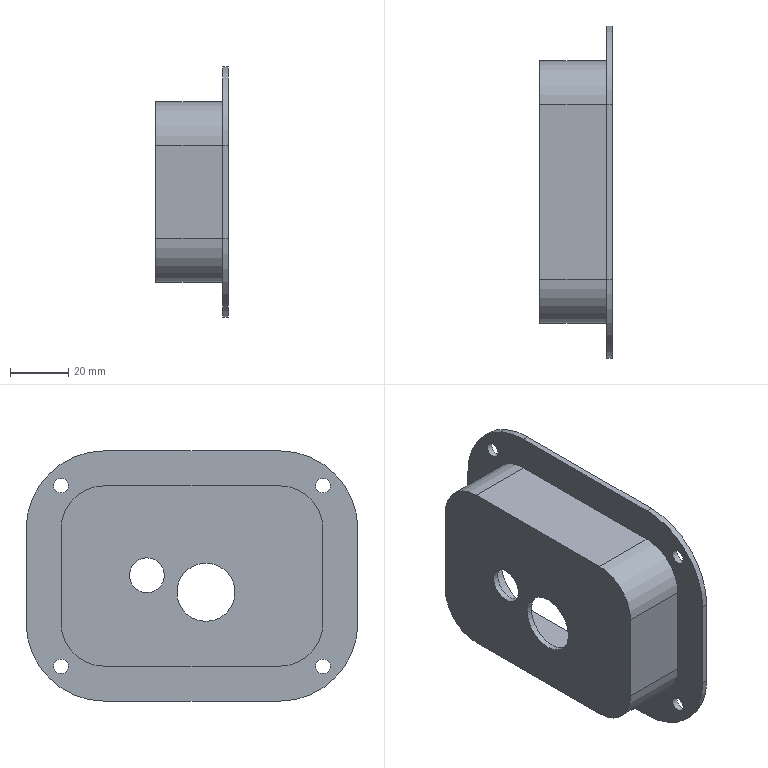Part | STEP file | Plug | 1 solid | 34 faces | box 25 x 114 x 86 mm | volume 29855 mm3 | cylinder 18 | plane 16 | commonest cylinder face diameters 5 x4 26 x4 30 x4 54 x4 12 x1 20 x1
STEP:
#1=CARTESIAN_POINT('',(23.,102.,-15.));
#2=VERTEX_POINT('',#1);
#3=CARTESIAN_POINT('',(23.,75.,12.));
#4=VERTEX_POINT('',#3);
#5=CARTESIAN_POINT('',(23.,75.,-15.));
#6=DIRECTION('',(1.,0.,0.));
#7=DIRECTION('',(0.,1.,0.));
#8=AXIS2_PLACEMENT_3D('',#5,#6,#7);
#9=CIRCLE('',#8,27.);
#10=EDGE_CURVE('',#2,#4,#9,.T.);
#11=ORIENTED_EDGE('',*,*,#10,.F.);
#12=CARTESIAN_POINT('',(23.,102.,-47.));
#13=VERTEX_POINT('',#12);
#14=CARTESIAN_POINT('',(23.,102.,-47.));
#15=DIRECTION('',(0.,0.,1.));
#16=VECTOR('',#15,1.);
#17=LINE('',#14,#16);
#18=EDGE_CURVE('',#13,#2,#17,.T.);
#19=ORIENTED_EDGE('',*,*,#18,.F.);
#20=CARTESIAN_POINT('',(23.,75.,-74.));
#21=VERTEX_POINT('',#20);
#22=CARTESIAN_POINT('',(23.,75.,-47.));
#23=DIRECTION('',(1.,0.,0.));
#24=DIRECTION('',(0.,0.,-1.));
#25=AXIS2_PLACEMENT_3D('',#22,#23,#24);
#26=CIRCLE('',#25,27.);
#27=EDGE_CURVE('',#21,#13,#26,.T.);
#28=ORIENTED_EDGE('',*,*,#27,.F.);
#29=CARTESIAN_POINT('',(23.,15.,-74.));
#30=VERTEX_POINT('',#29);
#31=CARTESIAN_POINT('',(23.,15.,-74.));
#32=DIRECTION('',(0.,1.,0.));
#33=VECTOR('',#32,1.);
#34=LINE('',#31,#33);
#35=EDGE_CURVE('',#30,#21,#34,.T.);
#36=ORIENTED_EDGE('',*,*,#35,.F.);
#37=CARTESIAN_POINT('',(23.,-12.,-47.));
#38=VERTEX_POINT('',#37);
#39=CARTESIAN_POINT('',(23.,15.,-47.));
#40=DIRECTION('',(1.,0.,0.));
#41=DIRECTION('',(0.,-1.,0.));
#42=AXIS2_PLACEMENT_3D('',#39,#40,#41);
#43=CIRCLE('',#42,27.);
#44=EDGE_CURVE('',#38,#30,#43,.T.);
#45=ORIENTED_EDGE('',*,*,#44,.F.);
#46=CARTESIAN_POINT('',(23.,-12.,-15.));
#47=VERTEX_POINT('',#46);
#48=CARTESIAN_POINT('',(23.,-12.,-15.));
#49=DIRECTION('',(0.,0.,-1.));
#50=VECTOR('',#49,1.);
#51=LINE('',#48,#50);
#52=EDGE_CURVE('',#47,#38,#51,.T.);
#53=ORIENTED_EDGE('',*,*,#52,.F.);
#54=CARTESIAN_POINT('',(23.,15.,12.));
#55=VERTEX_POINT('',#54);
#56=CARTESIAN_POINT('',(23.,15.,-15.));
#57=DIRECTION('',(1.,0.,0.));
#58=DIRECTION('',(0.,0.,1.));
#59=AXIS2_PLACEMENT_3D('',#56,#57,#58);
#60=CIRCLE('',#59,27.);
#61=EDGE_CURVE('',#55,#47,#60,.T.);
#62=ORIENTED_EDGE('',*,*,#61,.F.);
#63=CARTESIAN_POINT('',(23.,75.,12.));
#64=DIRECTION('',(0.,-1.,0.));
#65=VECTOR('',#64,1.);
#66=LINE('',#63,#65);
#67=EDGE_CURVE('',#4,#55,#66,.T.);
#68=ORIENTED_EDGE('',*,*,#67,.F.);
#69=EDGE_LOOP('',(#11,#19,#28,#36,#45,#53,#62,#68));
#70=FACE_BOUND('',#69,.T.);
#71=CARTESIAN_POINT('',(23.,92.5,-62.));
#72=VERTEX_POINT('',#71);
#73=CARTESIAN_POINT('',(23.,90.,-62.));
#74=DIRECTION('',(1.,0.,0.));
#75=DIRECTION('',(0.,1.,0.));
#76=AXIS2_PLACEMENT_3D('',#73,#74,#75);
#77=CIRCLE('',#76,2.5);
#78=EDGE_CURVE('',#72,#72,#77,.T.);
#79=ORIENTED_EDGE('',*,*,#78,.T.);
#80=EDGE_LOOP('',(#79));
#81=FACE_BOUND('',#80,.T.);
#82=CARTESIAN_POINT('',(23.,2.5,-62.));
#83=VERTEX_POINT('',#82);
#84=CARTESIAN_POINT('',(23.,0.,-62.));
#85=DIRECTION('',(1.,0.,0.));
#86=DIRECTION('',(0.,1.,0.));
#87=AXIS2_PLACEMENT_3D('',#84,#85,#86);
#88=CIRCLE('',#87,2.5);
#89=EDGE_CURVE('',#83,#83,#88,.T.);
#90=ORIENTED_EDGE('',*,*,#89,.T.);
#91=EDGE_LOOP('',(#90));
#92=FACE_BOUND('',#91,.T.);
#93=CARTESIAN_POINT('',(23.,2.5,0.));
#94=VERTEX_POINT('',#93);
#95=CARTESIAN_POINT('',(23.,0.,0.));
#96=DIRECTION('',(1.,0.,0.));
#97=DIRECTION('',(0.,1.,0.));
#98=AXIS2_PLACEMENT_3D('',#95,#96,#97);
#99=CIRCLE('',#98,2.5);
#100=EDGE_CURVE('',#94,#94,#99,.T.);
#101=ORIENTED_EDGE('',*,*,#100,.T.);
#102=EDGE_LOOP('',(#101));
#103=FACE_BOUND('',#102,.T.);
#104=CARTESIAN_POINT('',(23.,0.,-47.));
#105=VERTEX_POINT('',#104);
#106=CARTESIAN_POINT('',(23.,15.,-62.));
#107=VERTEX_POINT('',#106);
#108=CARTESIAN_POINT('',(23.,15.,-47.));
#109=DIRECTION('',(-1.,0.,0.));
#110=DIRECTION('',(0.,0.,-1.));
#111=AXIS2_PLACEMENT_3D('',#108,#109,#110);
#112=CIRCLE('',#111,15.);
#113=EDGE_CURVE('',#105,#107,#112,.F.);
#114=ORIENTED_EDGE('',*,*,#113,.T.);
#115=CARTESIAN_POINT('',(23.,75.,-62.));
#116=VERTEX_POINT('',#115);
#117=CARTESIAN_POINT('',(23.,75.,-62.));
#118=DIRECTION('',(0.,-1.,0.));
#119=VECTOR('',#118,1.);
#120=LINE('',#117,#119);
#121=EDGE_CURVE('',#107,#116,#120,.F.);
#122=ORIENTED_EDGE('',*,*,#121,.T.);
#123=CARTESIAN_POINT('',(23.,90.,-47.));
#124=VERTEX_POINT('',#123);
#125=CARTESIAN_POINT('',(23.,75.,-47.));
#126=DIRECTION('',(-1.,0.,0.));
#127=DIRECTION('',(0.,1.,0.));
#128=AXIS2_PLACEMENT_3D('',#125,#126,#127);
#129=CIRCLE('',#128,15.);
#130=EDGE_CURVE('',#116,#124,#129,.F.);
#131=ORIENTED_EDGE('',*,*,#130,.T.);
#132=CARTESIAN_POINT('',(23.,90.,-15.));
#133=VERTEX_POINT('',#132);
#134=CARTESIAN_POINT('',(23.,90.,-15.));
#135=DIRECTION('',(0.,0.,-1.));
#136=VECTOR('',#135,1.);
#137=LINE('',#134,#136);
#138=EDGE_CURVE('',#124,#133,#137,.F.);
#139=ORIENTED_EDGE('',*,*,#138,.T.);
#140=CARTESIAN_POINT('',(23.,75.,0.));
#141=VERTEX_POINT('',#140);
#142=CARTESIAN_POINT('',(23.,75.,-15.));
#143=DIRECTION('',(-1.,0.,0.));
#144=DIRECTION('',(0.,0.,1.));
#145=AXIS2_PLACEMENT_3D('',#142,#143,#144);
#146=CIRCLE('',#145,15.);
#147=EDGE_CURVE('',#133,#141,#146,.F.);
#148=ORIENTED_EDGE('',*,*,#147,.T.);
#149=CARTESIAN_POINT('',(23.,15.,0.));
#150=VERTEX_POINT('',#149);
#151=CARTESIAN_POINT('',(23.,15.,0.));
#152=DIRECTION('',(0.,1.,0.));
#153=VECTOR('',#152,1.);
#154=LINE('',#151,#153);
#155=EDGE_CURVE('',#141,#150,#154,.F.);
#156=ORIENTED_EDGE('',*,*,#155,.T.);
#157=CARTESIAN_POINT('',(23.,0.,-15.));
#158=VERTEX_POINT('',#157);
#159=CARTESIAN_POINT('',(23.,15.,-15.));
#160=DIRECTION('',(-1.,0.,0.));
#161=DIRECTION('',(0.,-1.,0.));
#162=AXIS2_PLACEMENT_3D('',#159,#160,#161);
#163=CIRCLE('',#162,15.);
#164=EDGE_CURVE('',#150,#158,#163,.F.);
#165=ORIENTED_EDGE('',*,*,#164,.T.);
#166=CARTESIAN_POINT('',(23.,0.,-47.));
#167=DIRECTION('',(0.,0.,1.));
#168=VECTOR('',#167,1.);
#169=LINE('',#166,#168);
#170=EDGE_CURVE('',#158,#105,#169,.F.);
#171=ORIENTED_EDGE('',*,*,#170,.T.);
#172=EDGE_LOOP('',(#114,#122,#131,#139,#148,#156,#165,#171));
#173=FACE_BOUND('',#172,.T.);
#174=CARTESIAN_POINT('',(23.,92.5,0.));
#175=VERTEX_POINT('',#174);
#176=CARTESIAN_POINT('',(23.,90.,0.));
#177=DIRECTION('',(1.,0.,0.));
#178=DIRECTION('',(0.,1.,0.));
#179=AXIS2_PLACEMENT_3D('',#176,#177,#178);
#180=CIRCLE('',#179,2.5);
#181=EDGE_CURVE('',#175,#175,#180,.T.);
#182=ORIENTED_EDGE('',*,*,#181,.T.);
#183=EDGE_LOOP('',(#182));
#184=FACE_BOUND('',#183,.T.);
#185=CARTESIAN_POINT('',(23.,0.,0.));
#186=DIRECTION('',(1.,0.,0.));
#187=DIRECTION('',(0.,0.,-1.));
#188=AXIS2_PLACEMENT_3D('',#185,#186,#187);
#189=PLANE('',#188);
#190=ADVANCED_FACE('',(#70,#81,#92,#103,#173,#184),#189,.F.);
#191=CARTESIAN_POINT('',(25.,75.,12.));
#192=VERTEX_POINT('',#191);
#193=CARTESIAN_POINT('',(25.,15.,12.));
#194=VERTEX_POINT('',#193);
#195=CARTESIAN_POINT('',(25.,75.,12.));
#196=DIRECTION('',(0.,-1.,0.));
#197=VECTOR('',#196,1.);
#198=LINE('',#195,#197);
#199=EDGE_CURVE('',#192,#194,#198,.T.);
#200=ORIENTED_EDGE('',*,*,#199,.T.);
#201=CARTESIAN_POINT('',(25.,-12.,-15.));
#202=VERTEX_POINT('',#201);
#203=CARTESIAN_POINT('',(25.,15.,-15.));
#204=DIRECTION('',(1.,0.,0.));
#205=DIRECTION('',(0.,0.,1.));
#206=AXIS2_PLACEMENT_3D('',#203,#204,#205);
#207=CIRCLE('',#206,27.);
#208=EDGE_CURVE('',#194,#202,#207,.T.);
#209=ORIENTED_EDGE('',*,*,#208,.T.);
#210=CARTESIAN_POINT('',(25.,-12.,-47.));
#211=VERTEX_POINT('',#210);
#212=CARTESIAN_POINT('',(25.,-12.,-15.));
#213=DIRECTION('',(0.,0.,-1.));
#214=VECTOR('',#213,1.);
#215=LINE('',#212,#214);
#216=EDGE_CURVE('',#202,#211,#215,.T.);
#217=ORIENTED_EDGE('',*,*,#216,.T.);
#218=CARTESIAN_POINT('',(25.,15.,-74.));
#219=VERTEX_POINT('',#218);
#220=CARTESIAN_POINT('',(25.,15.,-47.));
#221=DIRECTION('',(1.,0.,0.));
#222=DIRECTION('',(0.,-1.,0.));
#223=AXIS2_PLACEMENT_3D('',#220,#221,#222);
#224=CIRCLE('',#223,27.);
#225=EDGE_CURVE('',#211,#219,#224,.T.);
#226=ORIENTED_EDGE('',*,*,#225,.T.);
#227=CARTESIAN_POINT('',(25.,75.,-74.));
#228=VERTEX_POINT('',#227);
#229=CARTESIAN_POINT('',(25.,15.,-74.));
#230=DIRECTION('',(0.,1.,0.));
#231=VECTOR('',#230,1.);
#232=LINE('',#229,#231);
#233=EDGE_CURVE('',#219,#228,#232,.T.);
#234=ORIENTED_EDGE('',*,*,#233,.T.);
#235=CARTESIAN_POINT('',(25.,102.,-47.));
#236=VERTEX_POINT('',#235);
#237=CARTESIAN_POINT('',(25.,75.,-47.));
#238=DIRECTION('',(1.,0.,0.));
#239=DIRECTION('',(0.,0.,-1.));
#240=AXIS2_PLACEMENT_3D('',#237,#238,#239);
#241=CIRCLE('',#240,27.);
#242=EDGE_CURVE('',#228,#236,#241,.T.);
#243=ORIENTED_EDGE('',*,*,#242,.T.);
#244=CARTESIAN_POINT('',(25.,102.,-15.));
#245=VERTEX_POINT('',#244);
#246=CARTESIAN_POINT('',(25.,102.,-47.));
#247=DIRECTION('',(0.,0.,1.));
#248=VECTOR('',#247,1.);
#249=LINE('',#246,#248);
#250=EDGE_CURVE('',#236,#245,#249,.T.);
#251=ORIENTED_EDGE('',*,*,#250,.T.);
#252=CARTESIAN_POINT('',(25.,75.,-15.));
#253=DIRECTION('',(1.,0.,0.));
#254=DIRECTION('',(0.,1.,0.));
#255=AXIS2_PLACEMENT_3D('',#252,#253,#254);
#256=CIRCLE('',#255,27.);
#257=EDGE_CURVE('',#245,#192,#256,.T.);
#258=ORIENTED_EDGE('',*,*,#257,.T.);
#259=EDGE_LOOP('',(#200,#209,#217,#226,#234,#243,#251,#258));
#260=FACE_BOUND('',#259,.T.);
#261=CARTESIAN_POINT('',(25.,92.5,-62.));
#262=VERTEX_POINT('',#261);
#263=CARTESIAN_POINT('',(25.,90.,-62.));
#264=DIRECTION('',(1.,0.,0.));
#265=DIRECTION('',(0.,1.,0.));
#266=AXIS2_PLACEMENT_3D('',#263,#264,#265);
#267=CIRCLE('',#266,2.5);
#268=EDGE_CURVE('',#262,#262,#267,.F.);
#269=ORIENTED_EDGE('',*,*,#268,.T.);
#270=EDGE_LOOP('',(#269));
#271=FACE_BOUND('',#270,.T.);
#272=CARTESIAN_POINT('',(25.,2.5,-62.));
#273=VERTEX_POINT('',#272);
#274=CARTESIAN_POINT('',(25.,0.,-62.));
#275=DIRECTION('',(1.,0.,0.));
#276=DIRECTION('',(0.,1.,0.));
#277=AXIS2_PLACEMENT_3D('',#274,#275,#276);
#278=CIRCLE('',#277,2.5);
#279=EDGE_CURVE('',#273,#273,#278,.F.);
#280=ORIENTED_EDGE('',*,*,#279,.T.);
#281=EDGE_LOOP('',(#280));
#282=FACE_BOUND('',#281,.T.);
#283=CARTESIAN_POINT('',(25.,2.5,0.));
#284=VERTEX_POINT('',#283);
#285=CARTESIAN_POINT('',(25.,0.,0.));
#286=DIRECTION('',(1.,0.,0.));
#287=DIRECTION('',(0.,1.,0.));
#288=AXIS2_PLACEMENT_3D('',#285,#286,#287);
#289=CIRCLE('',#288,2.5);
#290=EDGE_CURVE('',#284,#284,#289,.F.);
#291=ORIENTED_EDGE('',*,*,#290,.T.);
#292=EDGE_LOOP('',(#291));
#293=FACE_BOUND('',#292,.T.);
#294=CARTESIAN_POINT('',(25.,75.,-2.));
#295=VERTEX_POINT('',#294);
#296=CARTESIAN_POINT('',(25.,88.,-15.));
#297=VERTEX_POINT('',#296);
#298=CARTESIAN_POINT('',(25.,75.,-15.));
#299=DIRECTION('',(1.,0.,0.));
#300=DIRECTION('',(0.,1.,0.));
#301=AXIS2_PLACEMENT_3D('',#298,#299,#300);
#302=CIRCLE('',#301,13.);
#303=EDGE_CURVE('',#295,#297,#302,.F.);
#304=ORIENTED_EDGE('',*,*,#303,.T.);
#305=CARTESIAN_POINT('',(25.,88.,-47.));
#306=VERTEX_POINT('',#305);
#307=CARTESIAN_POINT('',(25.,88.,-47.));
#308=DIRECTION('',(0.,0.,1.));
#309=VECTOR('',#308,1.);
#310=LINE('',#307,#309);
#311=EDGE_CURVE('',#297,#306,#310,.F.);
#312=ORIENTED_EDGE('',*,*,#311,.T.);
#313=CARTESIAN_POINT('',(25.,75.,-60.));
#314=VERTEX_POINT('',#313);
#315=CARTESIAN_POINT('',(25.,75.,-47.));
#316=DIRECTION('',(1.,0.,0.));
#317=DIRECTION('',(0.,0.,-1.));
#318=AXIS2_PLACEMENT_3D('',#315,#316,#317);
#319=CIRCLE('',#318,13.);
#320=EDGE_CURVE('',#306,#314,#319,.F.);
#321=ORIENTED_EDGE('',*,*,#320,.T.);
#322=CARTESIAN_POINT('',(25.,15.,-60.));
#323=VERTEX_POINT('',#322);
#324=CARTESIAN_POINT('',(25.,15.,-60.));
#325=DIRECTION('',(0.,1.,0.));
#326=VECTOR('',#325,1.);
#327=LINE('',#324,#326);
#328=EDGE_CURVE('',#314,#323,#327,.F.);
#329=ORIENTED_EDGE('',*,*,#328,.T.);
#330=CARTESIAN_POINT('',(25.,2.,-47.));
#331=VERTEX_POINT('',#330);
#332=CARTESIAN_POINT('',(25.,15.,-47.));
#333=DIRECTION('',(1.,0.,0.));
#334=DIRECTION('',(0.,-1.,0.));
#335=AXIS2_PLACEMENT_3D('',#332,#333,#334);
#336=CIRCLE('',#335,13.);
#337=EDGE_CURVE('',#323,#331,#336,.F.);
#338=ORIENTED_EDGE('',*,*,#337,.T.);
#339=CARTESIAN_POINT('',(25.,2.,-15.));
#340=VERTEX_POINT('',#339);
#341=CARTESIAN_POINT('',(25.,2.,-15.));
#342=DIRECTION('',(0.,0.,-1.));
#343=VECTOR('',#342,1.);
#344=LINE('',#341,#343);
#345=EDGE_CURVE('',#331,#340,#344,.F.);
#346=ORIENTED_EDGE('',*,*,#345,.T.);
#347=CARTESIAN_POINT('',(25.,15.,-2.));
#348=VERTEX_POINT('',#347);
#349=CARTESIAN_POINT('',(25.,15.,-15.));
#350=DIRECTION('',(1.,0.,0.));
#351=DIRECTION('',(0.,0.,1.));
#352=AXIS2_PLACEMENT_3D('',#349,#350,#351);
#353=CIRCLE('',#352,13.);
#354=EDGE_CURVE('',#340,#348,#353,.F.);
#355=ORIENTED_EDGE('',*,*,#354,.T.);
#356=CARTESIAN_POINT('',(25.,75.,-2.));
#357=DIRECTION('',(0.,-1.,0.));
#358=VECTOR('',#357,1.);
#359=LINE('',#356,#358);
#360=EDGE_CURVE('',#348,#295,#359,.F.);
#361=ORIENTED_EDGE('',*,*,#360,.T.);
#362=EDGE_LOOP('',(#304,#312,#321,#329,#338,#346,#355,#361));
#363=FACE_BOUND('',#362,.T.);
#364=CARTESIAN_POINT('',(25.,92.5,0.));
#365=VERTEX_POINT('',#364);
#366=CARTESIAN_POINT('',(25.,90.,0.));
#367=DIRECTION('',(1.,0.,0.));
#368=DIRECTION('',(0.,1.,0.));
#369=AXIS2_PLACEMENT_3D('',#366,#367,#368);
#370=CIRCLE('',#369,2.5);
#371=EDGE_CURVE('',#365,#365,#370,.F.);
#372=ORIENTED_EDGE('',*,*,#371,.T.);
#373=EDGE_LOOP('',(#372));
#374=FACE_BOUND('',#373,.T.);
#375=CARTESIAN_POINT('',(25.,0.,0.));
#376=DIRECTION('',(1.,0.,0.));
#377=DIRECTION('',(0.,0.,-1.));
#378=AXIS2_PLACEMENT_3D('',#375,#376,#377);
#379=PLANE('',#378);
#380=ADVANCED_FACE('',(#260,#271,#282,#293,#363,#374),#379,.T.);
#381=ORIENTED_EDGE('',*,*,#290,.F.);
#382=EDGE_LOOP('',(#381));
#383=FACE_OUTER_BOUND('',#382,.T.);
#384=ORIENTED_EDGE('',*,*,#100,.F.);
#385=EDGE_LOOP('',(#384));
#386=FACE_OUTER_BOUND('',#385,.T.);
#387=CARTESIAN_POINT('',(-15.,0.,0.));
#388=DIRECTION('',(1.,0.,0.));
#389=DIRECTION('',(0.,1.,0.));
#390=AXIS2_PLACEMENT_3D('',#387,#388,#389);
#391=CYLINDRICAL_SURFACE('',#390,2.5);
#392=ADVANCED_FACE('',(#383,#386),#391,.F.);
#393=ORIENTED_EDGE('',*,*,#279,.F.);
#394=EDGE_LOOP('',(#393));
#395=FACE_OUTER_BOUND('',#394,.T.);
#396=ORIENTED_EDGE('',*,*,#89,.F.);
#397=EDGE_LOOP('',(#396));
#398=FACE_OUTER_BOUND('',#397,.T.);
#399=CARTESIAN_POINT('',(-15.,0.,-62.));
#400=DIRECTION('',(1.,0.,0.));
#401=DIRECTION('',(0.,1.,0.));
#402=AXIS2_PLACEMENT_3D('',#399,#400,#401);
#403=CYLINDRICAL_SURFACE('',#402,2.5);
#404=ADVANCED_FACE('',(#395,#398),#403,.F.);
#405=ORIENTED_EDGE('',*,*,#268,.F.);
#406=EDGE_LOOP('',(#405));
#407=FACE_OUTER_BOUND('',#406,.T.);
#408=ORIENTED_EDGE('',*,*,#78,.F.);
#409=EDGE_LOOP('',(#408));
#410=FACE_OUTER_BOUND('',#409,.T.);
#411=CARTESIAN_POINT('',(-15.,90.,-62.));
#412=DIRECTION('',(1.,0.,0.));
#413=DIRECTION('',(0.,1.,0.));
#414=AXIS2_PLACEMENT_3D('',#411,#412,#413);
#415=CYLINDRICAL_SURFACE('',#414,2.5);
#416=ADVANCED_FACE('',(#407,#410),#415,.F.);
#417=ORIENTED_EDGE('',*,*,#10,.T.);
#418=CARTESIAN_POINT('',(23.,75.,12.));
#419=DIRECTION('',(1.,0.,0.));
#420=VECTOR('',#419,1.);
#421=LINE('',#418,#420);
#422=EDGE_CURVE('',#4,#192,#421,.T.);
#423=ORIENTED_EDGE('',*,*,#422,.T.);
#424=ORIENTED_EDGE('',*,*,#257,.F.);
#425=CARTESIAN_POINT('',(23.,102.,-15.));
#426=DIRECTION('',(1.,0.,0.));
#427=VECTOR('',#426,1.);
#428=LINE('',#425,#427);
#429=EDGE_CURVE('',#2,#245,#428,.T.);
#430=ORIENTED_EDGE('',*,*,#429,.F.);
#431=EDGE_LOOP('',(#417,#423,#424,#430));
#432=FACE_BOUND('',#431,.T.);
#433=CARTESIAN_POINT('',(23.,75.,-15.));
#434=DIRECTION('',(1.,0.,0.));
#435=DIRECTION('',(0.,1.,0.));
#436=AXIS2_PLACEMENT_3D('',#433,#434,#435);
#437=CYLINDRICAL_SURFACE('',#436,27.);
#438=ADVANCED_FACE('',(#432),#437,.T.);
#439=ORIENTED_EDGE('',*,*,#18,.T.);
#440=ORIENTED_EDGE('',*,*,#429,.T.);
#441=ORIENTED_EDGE('',*,*,#250,.F.);
#442=CARTESIAN_POINT('',(23.,102.,-47.));
#443=DIRECTION('',(1.,0.,0.));
#444=VECTOR('',#443,1.);
#445=LINE('',#442,#444);
#446=EDGE_CURVE('',#13,#236,#445,.T.);
#447=ORIENTED_EDGE('',*,*,#446,.F.);
#448=EDGE_LOOP('',(#439,#440,#441,#447));
#449=FACE_BOUND('',#448,.T.);
#450=CARTESIAN_POINT('',(23.,102.,-47.));
#451=DIRECTION('',(0.,1.,0.));
#452=DIRECTION('',(0.,0.,1.));
#453=AXIS2_PLACEMENT_3D('',#450,#451,#452);
#454=PLANE('',#453);
#455=ADVANCED_FACE('',(#449),#454,.T.);
#456=ORIENTED_EDGE('',*,*,#27,.T.);
#457=ORIENTED_EDGE('',*,*,#446,.T.);
#458=ORIENTED_EDGE('',*,*,#242,.F.);
#459=CARTESIAN_POINT('',(23.,75.,-74.));
#460=DIRECTION('',(1.,0.,0.));
#461=VECTOR('',#460,1.);
#462=LINE('',#459,#461);
#463=EDGE_CURVE('',#21,#228,#462,.T.);
#464=ORIENTED_EDGE('',*,*,#463,.F.);
#465=EDGE_LOOP('',(#456,#457,#458,#464));
#466=FACE_BOUND('',#465,.T.);
#467=CARTESIAN_POINT('',(23.,75.,-47.));
#468=DIRECTION('',(1.,0.,0.));
#469=DIRECTION('',(0.,0.,-1.));
#470=AXIS2_PLACEMENT_3D('',#467,#468,#469);
#471=CYLINDRICAL_SURFACE('',#470,27.);
#472=ADVANCED_FACE('',(#466),#471,.T.);
#473=ORIENTED_EDGE('',*,*,#35,.T.);
#474=ORIENTED_EDGE('',*,*,#463,.T.);
#475=ORIENTED_EDGE('',*,*,#233,.F.);
#476=CARTESIAN_POINT('',(23.,15.,-74.));
#477=DIRECTION('',(1.,0.,0.));
#478=VECTOR('',#477,1.);
#479=LINE('',#476,#478);
#480=EDGE_CURVE('',#30,#219,#479,.T.);
#481=ORIENTED_EDGE('',*,*,#480,.F.);
#482=EDGE_LOOP('',(#473,#474,#475,#481));
#483=FACE_BOUND('',#482,.T.);
#484=CARTESIAN_POINT('',(23.,15.,-74.));
#485=DIRECTION('',(0.,0.,-1.));
#486=DIRECTION('',(0.,1.,0.));
#487=AXIS2_PLACEMENT_3D('',#484,#485,#486);
#488=PLANE('',#487);
#489=ADVANCED_FACE('',(#483),#488,.T.);
#490=ORIENTED_EDGE('',*,*,#44,.T.);
#491=ORIENTED_EDGE('',*,*,#480,.T.);
#492=ORIENTED_EDGE('',*,*,#225,.F.);
#493=CARTESIAN_POINT('',(23.,-12.,-47.));
#494=DIRECTION('',(1.,0.,0.));
#495=VECTOR('',#494,1.);
#496=LINE('',#493,#495);
#497=EDGE_CURVE('',#38,#211,#496,.T.);
#498=ORIENTED_EDGE('',*,*,#497,.F.);
#499=EDGE_LOOP('',(#490,#491,#492,#498));
#500=FACE_BOUND('',#499,.T.);
#501=CARTESIAN_POINT('',(23.,15.,-47.));
#502=DIRECTION('',(1.,0.,0.));
#503=DIRECTION('',(0.,-1.,0.));
#504=AXIS2_PLACEMENT_3D('',#501,#502,#503);
#505=CYLINDRICAL_SURFACE('',#504,27.);
#506=ADVANCED_FACE('',(#500),#505,.T.);
#507=ORIENTED_EDGE('',*,*,#52,.T.);
#508=ORIENTED_EDGE('',*,*,#497,.T.);
#509=ORIENTED_EDGE('',*,*,#216,.F.);
#510=CARTESIAN_POINT('',(23.,-12.,-15.));
#511=DIRECTION('',(1.,0.,0.));
#512=VECTOR('',#511,1.);
#513=LINE('',#510,#512);
#514=EDGE_CURVE('',#47,#202,#513,.T.);
#515=ORIENTED_EDGE('',*,*,#514,.F.);
#516=EDGE_LOOP('',(#507,#508,#509,#515));
#517=FACE_BOUND('',#516,.T.);
#518=CARTESIAN_POINT('',(23.,-12.,-15.));
#519=DIRECTION('',(0.,-1.,0.));
#520=DIRECTION('',(0.,0.,-1.));
#521=AXIS2_PLACEMENT_3D('',#518,#519,#520);
#522=PLANE('',#521);
#523=ADVANCED_FACE('',(#517),#522,.T.);
#524=ORIENTED_EDGE('',*,*,#61,.T.);
#525=ORIENTED_EDGE('',*,*,#514,.T.);
#526=ORIENTED_EDGE('',*,*,#208,.F.);
#527=CARTESIAN_POINT('',(23.,15.,12.));
#528=DIRECTION('',(1.,0.,0.));
#529=VECTOR('',#528,1.);
#530=LINE('',#527,#529);
#531=EDGE_CURVE('',#55,#194,#530,.T.);
#532=ORIENTED_EDGE('',*,*,#531,.F.);
#533=EDGE_LOOP('',(#524,#525,#526,#532));
#534=FACE_BOUND('',#533,.T.);
#535=CARTESIAN_POINT('',(23.,15.,-15.));
#536=DIRECTION('',(1.,0.,0.));
#537=DIRECTION('',(0.,0.,1.));
#538=AXIS2_PLACEMENT_3D('',#535,#536,#537);
#539=CYLINDRICAL_SURFACE('',#538,27.);
#540=ADVANCED_FACE('',(#534),#539,.T.);
#541=ORIENTED_EDGE('',*,*,#67,.T.);
#542=ORIENTED_EDGE('',*,*,#531,.T.);
#543=ORIENTED_EDGE('',*,*,#199,.F.);
#544=ORIENTED_EDGE('',*,*,#422,.F.);
#545=EDGE_LOOP('',(#541,#542,#543,#544));
#546=FACE_BOUND('',#545,.T.);
#547=CARTESIAN_POINT('',(23.,75.,12.));
#548=DIRECTION('',(0.,0.,1.));
#549=DIRECTION('',(0.,-1.,0.));
#550=AXIS2_PLACEMENT_3D('',#547,#548,#549);
#551=PLANE('',#550);
#552=ADVANCED_FACE('',(#546),#551,.T.);
#553=ORIENTED_EDGE('',*,*,#113,.F.);
#554=CARTESIAN_POINT('',(0.,0.,-47.));
#555=VERTEX_POINT('',#554);
#556=CARTESIAN_POINT('',(0.,0.,-47.));
#557=DIRECTION('',(1.,0.,0.));
#558=VECTOR('',#557,1.);
#559=LINE('',#556,#558);
#560=EDGE_CURVE('',#555,#105,#559,.T.);
#561=ORIENTED_EDGE('',*,*,#560,.F.);
#562=CARTESIAN_POINT('',(0.,15.,-62.));
#563=VERTEX_POINT('',#562);
#564=CARTESIAN_POINT('',(0.,15.,-47.));
#565=DIRECTION('',(-1.,0.,0.));
#566=DIRECTION('',(0.,0.,-1.));
#567=AXIS2_PLACEMENT_3D('',#564,#565,#566);
#568=CIRCLE('',#567,15.);
#569=EDGE_CURVE('',#555,#563,#568,.F.);
#570=ORIENTED_EDGE('',*,*,#569,.T.);
#571=CARTESIAN_POINT('',(0.,15.,-62.));
#572=DIRECTION('',(1.,0.,0.));
#573=VECTOR('',#572,1.);
#574=LINE('',#571,#573);
#575=EDGE_CURVE('',#563,#107,#574,.T.);
#576=ORIENTED_EDGE('',*,*,#575,.T.);
#577=EDGE_LOOP('',(#553,#561,#570,#576));
#578=FACE_BOUND('',#577,.T.);
#579=CARTESIAN_POINT('',(-60.,15.,-47.));
#580=DIRECTION('',(-1.,0.,0.));
#581=DIRECTION('',(0.,0.,-1.));
#582=AXIS2_PLACEMENT_3D('',#579,#580,#581);
#583=CYLINDRICAL_SURFACE('',#582,15.);
#584=ADVANCED_FACE('',(#578),#583,.T.);
#585=ORIENTED_EDGE('',*,*,#121,.F.);
#586=ORIENTED_EDGE('',*,*,#575,.F.);
#587=CARTESIAN_POINT('',(0.,75.,-62.));
#588=VERTEX_POINT('',#587);
#589=CARTESIAN_POINT('',(0.,15.,-62.));
#590=DIRECTION('',(0.,1.,0.));
#591=VECTOR('',#590,1.);
#592=LINE('',#589,#591);
#593=EDGE_CURVE('',#563,#588,#592,.T.);
#594=ORIENTED_EDGE('',*,*,#593,.T.);
#595=CARTESIAN_POINT('',(0.,75.,-62.));
#596=DIRECTION('',(1.,0.,0.));
#597=VECTOR('',#596,1.);
#598=LINE('',#595,#597);
#599=EDGE_CURVE('',#588,#116,#598,.T.);
#600=ORIENTED_EDGE('',*,*,#599,.T.);
#601=EDGE_LOOP('',(#585,#586,#594,#600));
#602=FACE_BOUND('',#601,.T.);
#603=CARTESIAN_POINT('',(0.,0.,-62.));
#604=DIRECTION('',(0.,0.,-1.));
#605=DIRECTION('',(0.,1.,0.));
#606=AXIS2_PLACEMENT_3D('',#603,#604,#605);
#607=PLANE('',#606);
#608=ADVANCED_FACE('',(#602),#607,.T.);
#609=ORIENTED_EDGE('',*,*,#130,.F.);
#610=ORIENTED_EDGE('',*,*,#599,.F.);
#611=CARTESIAN_POINT('',(0.,90.,-47.));
#612=VERTEX_POINT('',#611);
#613=CARTESIAN_POINT('',(0.,75.,-47.));
#614=DIRECTION('',(-1.,0.,0.));
#615=DIRECTION('',(0.,1.,0.));
#616=AXIS2_PLACEMENT_3D('',#613,#614,#615);
#617=CIRCLE('',#616,15.);
#618=EDGE_CURVE('',#588,#612,#617,.F.);
#619=ORIENTED_EDGE('',*,*,#618,.T.);
#620=CARTESIAN_POINT('',(0.,90.,-47.));
#621=DIRECTION('',(1.,0.,0.));
#622=VECTOR('',#621,1.);
#623=LINE('',#620,#622);
#624=EDGE_CURVE('',#612,#124,#623,.T.);
#625=ORIENTED_EDGE('',*,*,#624,.T.);
#626=EDGE_LOOP('',(#609,#610,#619,#625));
#627=FACE_BOUND('',#626,.T.);
#628=CARTESIAN_POINT('',(-60.,75.,-47.));
#629=DIRECTION('',(-1.,0.,0.));
#630=DIRECTION('',(0.,1.,0.));
#631=AXIS2_PLACEMENT_3D('',#628,#629,#630);
#632=CYLINDRICAL_SURFACE('',#631,15.);
#633=ADVANCED_FACE('',(#627),#632,.T.);
#634=ORIENTED_EDGE('',*,*,#138,.F.);
#635=ORIENTED_EDGE('',*,*,#624,.F.);
#636=CARTESIAN_POINT('',(0.,90.,-15.));
#637=VERTEX_POINT('',#636);
#638=CARTESIAN_POINT('',(0.,90.,-47.));
#639=DIRECTION('',(0.,0.,1.));
#640=VECTOR('',#639,1.);
#641=LINE('',#638,#640);
#642=EDGE_CURVE('',#612,#637,#641,.T.);
#643=ORIENTED_EDGE('',*,*,#642,.T.);
#644=CARTESIAN_POINT('',(0.,90.,-15.));
#645=DIRECTION('',(1.,0.,0.));
#646=VECTOR('',#645,1.);
#647=LINE('',#644,#646);
#648=EDGE_CURVE('',#637,#133,#647,.T.);
#649=ORIENTED_EDGE('',*,*,#648,.T.);
#650=EDGE_LOOP('',(#634,#635,#643,#649));
#651=FACE_BOUND('',#650,.T.);
#652=CARTESIAN_POINT('',(0.,90.,-62.));
#653=DIRECTION('',(0.,1.,0.));
#654=DIRECTION('',(0.,0.,1.));
#655=AXIS2_PLACEMENT_3D('',#652,#653,#654);
#656=PLANE('',#655);
#657=ADVANCED_FACE('',(#651),#656,.T.);
#658=ORIENTED_EDGE('',*,*,#147,.F.);
#659=ORIENTED_EDGE('',*,*,#648,.F.);
#660=CARTESIAN_POINT('',(0.,75.,0.));
#661=VERTEX_POINT('',#660);
#662=CARTESIAN_POINT('',(0.,75.,-15.));
#663=DIRECTION('',(-1.,0.,0.));
#664=DIRECTION('',(0.,0.,1.));
#665=AXIS2_PLACEMENT_3D('',#662,#663,#664);
#666=CIRCLE('',#665,15.);
#667=EDGE_CURVE('',#637,#661,#666,.F.);
#668=ORIENTED_EDGE('',*,*,#667,.T.);
#669=CARTESIAN_POINT('',(0.,75.,0.));
#670=DIRECTION('',(1.,0.,0.));
#671=VECTOR('',#670,1.);
#672=LINE('',#669,#671);
#673=EDGE_CURVE('',#661,#141,#672,.T.);
#674=ORIENTED_EDGE('',*,*,#673,.T.);
#675=EDGE_LOOP('',(#658,#659,#668,#674));
#676=FACE_BOUND('',#675,.T.);
#677=CARTESIAN_POINT('',(-60.,75.,-15.));
#678=DIRECTION('',(-1.,0.,0.));
#679=DIRECTION('',(0.,0.,1.));
#680=AXIS2_PLACEMENT_3D('',#677,#678,#679);
#681=CYLINDRICAL_SURFACE('',#680,15.);
#682=ADVANCED_FACE('',(#676),#681,.T.);
#683=ORIENTED_EDGE('',*,*,#155,.F.);
#684=ORIENTED_EDGE('',*,*,#673,.F.);
#685=CARTESIAN_POINT('',(0.,15.,0.));
#686=VERTEX_POINT('',#685);
#687=CARTESIAN_POINT('',(0.,75.,0.));
#688=DIRECTION('',(0.,-1.,0.));
#689=VECTOR('',#688,1.);
#690=LINE('',#687,#689);
#691=EDGE_CURVE('',#661,#686,#690,.T.);
#692=ORIENTED_EDGE('',*,*,#691,.T.);
#693=CARTESIAN_POINT('',(0.,15.,0.));
#694=DIRECTION('',(1.,0.,0.));
#695=VECTOR('',#694,1.);
#696=LINE('',#693,#695);
#697=EDGE_CURVE('',#686,#150,#696,.T.);
#698=ORIENTED_EDGE('',*,*,#697,.T.);
#699=EDGE_LOOP('',(#683,#684,#692,#698));
#700=FACE_BOUND('',#699,.T.);
#701=CARTESIAN_POINT('',(0.,90.,0.));
#702=DIRECTION('',(0.,0.,1.));
#703=DIRECTION('',(0.,-1.,0.));
#704=AXIS2_PLACEMENT_3D('',#701,#702,#703);
#705=PLANE('',#704);
#706=ADVANCED_FACE('',(#700),#705,.T.);
#707=ORIENTED_EDGE('',*,*,#164,.F.);
#708=ORIENTED_EDGE('',*,*,#697,.F.);
#709=CARTESIAN_POINT('',(0.,0.,-15.));
#710=VERTEX_POINT('',#709);
#711=CARTESIAN_POINT('',(0.,15.,-15.));
#712=DIRECTION('',(-1.,0.,0.));
#713=DIRECTION('',(0.,-1.,0.));
#714=AXIS2_PLACEMENT_3D('',#711,#712,#713);
#715=CIRCLE('',#714,15.);
#716=EDGE_CURVE('',#686,#710,#715,.F.);
#717=ORIENTED_EDGE('',*,*,#716,.T.);
#718=CARTESIAN_POINT('',(0.,0.,-15.));
#719=DIRECTION('',(1.,0.,0.));
#720=VECTOR('',#719,1.);
#721=LINE('',#718,#720);
#722=EDGE_CURVE('',#710,#158,#721,.T.);
#723=ORIENTED_EDGE('',*,*,#722,.T.);
#724=EDGE_LOOP('',(#707,#708,#717,#723));
#725=FACE_BOUND('',#724,.T.);
#726=CARTESIAN_POINT('',(-60.,15.,-15.));
#727=DIRECTION('',(-1.,0.,0.));
#728=DIRECTION('',(0.,-1.,0.));
#729=AXIS2_PLACEMENT_3D('',#726,#727,#728);
#730=CYLINDRICAL_SURFACE('',#729,15.);
#731=ADVANCED_FACE('',(#725),#730,.T.);
#732=ORIENTED_EDGE('',*,*,#170,.F.);
#733=ORIENTED_EDGE('',*,*,#722,.F.);
#734=CARTESIAN_POINT('',(0.,0.,-15.));
#735=DIRECTION('',(0.,0.,-1.));
#736=VECTOR('',#735,1.);
#737=LINE('',#734,#736);
#738=EDGE_CURVE('',#710,#555,#737,.T.);
#739=ORIENTED_EDGE('',*,*,#738,.T.);
#740=ORIENTED_EDGE('',*,*,#560,.T.);
#741=EDGE_LOOP('',(#732,#733,#739,#740));
#742=FACE_BOUND('',#741,.T.);
#743=CARTESIAN_POINT('',(0.,0.,0.));
#744=DIRECTION('',(0.,-1.,0.));
#745=DIRECTION('',(0.,0.,-1.));
#746=AXIS2_PLACEMENT_3D('',#743,#744,#745);
#747=PLANE('',#746);
#748=ADVANCED_FACE('',(#742),#747,.T.);
#749=ORIENTED_EDGE('',*,*,#371,.F.);
#750=EDGE_LOOP('',(#749));
#751=FACE_OUTER_BOUND('',#750,.T.);
#752=ORIENTED_EDGE('',*,*,#181,.F.);
#753=EDGE_LOOP('',(#752));
#754=FACE_OUTER_BOUND('',#753,.T.);
#755=CARTESIAN_POINT('',(-15.,90.,0.));
#756=DIRECTION('',(1.,0.,0.));
#757=DIRECTION('',(0.,1.,0.));
#758=AXIS2_PLACEMENT_3D('',#755,#756,#757);
#759=CYLINDRICAL_SURFACE('',#758,2.5);
#760=ADVANCED_FACE('',(#751,#754),#759,.F.);
#761=CARTESIAN_POINT('',(2.,75.,-2.));
#762=VERTEX_POINT('',#761);
#763=CARTESIAN_POINT('',(2.,75.,-2.));
#764=DIRECTION('',(1.,0.,0.));
#765=VECTOR('',#764,1.);
#766=LINE('',#763,#765);
#767=EDGE_CURVE('',#762,#295,#766,.T.);
#768=ORIENTED_EDGE('',*,*,#767,.F.);
#769=CARTESIAN_POINT('',(2.,88.,-15.));
#770=VERTEX_POINT('',#769);
#771=CARTESIAN_POINT('',(2.,75.,-15.));
#772=DIRECTION('',(1.,0.,0.));
#773=DIRECTION('',(0.,1.,0.));
#774=AXIS2_PLACEMENT_3D('',#771,#772,#773);
#775=CIRCLE('',#774,13.);
#776=EDGE_CURVE('',#770,#762,#775,.T.);
#777=ORIENTED_EDGE('',*,*,#776,.F.);
#778=CARTESIAN_POINT('',(2.,88.,-15.));
#779=DIRECTION('',(1.,0.,0.));
#780=VECTOR('',#779,1.);
#781=LINE('',#778,#780);
#782=EDGE_CURVE('',#770,#297,#781,.T.);
#783=ORIENTED_EDGE('',*,*,#782,.T.);
#784=ORIENTED_EDGE('',*,*,#303,.F.);
#785=EDGE_LOOP('',(#768,#777,#783,#784));
#786=FACE_BOUND('',#785,.T.);
#787=CARTESIAN_POINT('',(2.,75.,-15.));
#788=DIRECTION('',(1.,0.,0.));
#789=DIRECTION('',(0.,1.,0.));
#790=AXIS2_PLACEMENT_3D('',#787,#788,#789);
#791=CYLINDRICAL_SURFACE('',#790,13.);
#792=ADVANCED_FACE('',(#786),#791,.F.);
#793=ORIENTED_EDGE('',*,*,#782,.F.);
#794=CARTESIAN_POINT('',(2.,88.,-47.));
#795=VERTEX_POINT('',#794);
#796=CARTESIAN_POINT('',(2.,88.,-47.));
#797=DIRECTION('',(0.,0.,1.));
#798=VECTOR('',#797,1.);
#799=LINE('',#796,#798);
#800=EDGE_CURVE('',#795,#770,#799,.T.);
#801=ORIENTED_EDGE('',*,*,#800,.F.);
#802=CARTESIAN_POINT('',(2.,88.,-47.));
#803=DIRECTION('',(1.,0.,0.));
#804=VECTOR('',#803,1.);
#805=LINE('',#802,#804);
#806=EDGE_CURVE('',#795,#306,#805,.T.);
#807=ORIENTED_EDGE('',*,*,#806,.T.);
#808=ORIENTED_EDGE('',*,*,#311,.F.);
#809=EDGE_LOOP('',(#793,#801,#807,#808));
#810=FACE_BOUND('',#809,.T.);
#811=CARTESIAN_POINT('',(2.,88.,-47.));
#812=DIRECTION('',(0.,1.,0.));
#813=DIRECTION('',(0.,0.,1.));
#814=AXIS2_PLACEMENT_3D('',#811,#812,#813);
#815=PLANE('',#814);
#816=ADVANCED_FACE('',(#810),#815,.F.);
#817=ORIENTED_EDGE('',*,*,#806,.F.);
#818=CARTESIAN_POINT('',(2.,75.,-60.));
#819=VERTEX_POINT('',#818);
#820=CARTESIAN_POINT('',(2.,75.,-47.));
#821=DIRECTION('',(1.,0.,0.));
#822=DIRECTION('',(0.,0.,-1.));
#823=AXIS2_PLACEMENT_3D('',#820,#821,#822);
#824=CIRCLE('',#823,13.);
#825=EDGE_CURVE('',#819,#795,#824,.T.);
#826=ORIENTED_EDGE('',*,*,#825,.F.);
#827=CARTESIAN_POINT('',(2.,75.,-60.));
#828=DIRECTION('',(1.,0.,0.));
#829=VECTOR('',#828,1.);
#830=LINE('',#827,#829);
#831=EDGE_CURVE('',#819,#314,#830,.T.);
#832=ORIENTED_EDGE('',*,*,#831,.T.);
#833=ORIENTED_EDGE('',*,*,#320,.F.);
#834=EDGE_LOOP('',(#817,#826,#832,#833));
#835=FACE_BOUND('',#834,.T.);
#836=CARTESIAN_POINT('',(2.,75.,-47.));
#837=DIRECTION('',(1.,0.,0.));
#838=DIRECTION('',(0.,0.,-1.));
#839=AXIS2_PLACEMENT_3D('',#836,#837,#838);
#840=CYLINDRICAL_SURFACE('',#839,13.);
#841=ADVANCED_FACE('',(#835),#840,.F.);
#842=ORIENTED_EDGE('',*,*,#831,.F.);
#843=CARTESIAN_POINT('',(2.,15.,-60.));
#844=VERTEX_POINT('',#843);
#845=CARTESIAN_POINT('',(2.,15.,-60.));
#846=DIRECTION('',(0.,1.,0.));
#847=VECTOR('',#846,1.);
#848=LINE('',#845,#847);
#849=EDGE_CURVE('',#844,#819,#848,.T.);
#850=ORIENTED_EDGE('',*,*,#849,.F.);
#851=CARTESIAN_POINT('',(2.,15.,-60.));
#852=DIRECTION('',(1.,0.,0.));
#853=VECTOR('',#852,1.);
#854=LINE('',#851,#853);
#855=EDGE_CURVE('',#844,#323,#854,.T.);
#856=ORIENTED_EDGE('',*,*,#855,.T.);
#857=ORIENTED_EDGE('',*,*,#328,.F.);
#858=EDGE_LOOP('',(#842,#850,#856,#857));
#859=FACE_BOUND('',#858,.T.);
#860=CARTESIAN_POINT('',(2.,15.,-60.));
#861=DIRECTION('',(0.,0.,-1.));
#862=DIRECTION('',(0.,1.,0.));
#863=AXIS2_PLACEMENT_3D('',#860,#861,#862);
#864=PLANE('',#863);
#865=ADVANCED_FACE('',(#859),#864,.F.);
#866=ORIENTED_EDGE('',*,*,#855,.F.);
#867=CARTESIAN_POINT('',(2.,2.,-47.));
#868=VERTEX_POINT('',#867);
#869=CARTESIAN_POINT('',(2.,15.,-47.));
#870=DIRECTION('',(1.,0.,0.));
#871=DIRECTION('',(0.,-1.,0.));
#872=AXIS2_PLACEMENT_3D('',#869,#870,#871);
#873=CIRCLE('',#872,13.);
#874=EDGE_CURVE('',#868,#844,#873,.T.);
#875=ORIENTED_EDGE('',*,*,#874,.F.);
#876=CARTESIAN_POINT('',(2.,2.,-47.));
#877=DIRECTION('',(1.,0.,0.));
#878=VECTOR('',#877,1.);
#879=LINE('',#876,#878);
#880=EDGE_CURVE('',#868,#331,#879,.T.);
#881=ORIENTED_EDGE('',*,*,#880,.T.);
#882=ORIENTED_EDGE('',*,*,#337,.F.);
#883=EDGE_LOOP('',(#866,#875,#881,#882));
#884=FACE_BOUND('',#883,.T.);
#885=CARTESIAN_POINT('',(2.,15.,-47.));
#886=DIRECTION('',(1.,0.,0.));
#887=DIRECTION('',(0.,-1.,0.));
#888=AXIS2_PLACEMENT_3D('',#885,#886,#887);
#889=CYLINDRICAL_SURFACE('',#888,13.);
#890=ADVANCED_FACE('',(#884),#889,.F.);
#891=ORIENTED_EDGE('',*,*,#880,.F.);
#892=CARTESIAN_POINT('',(2.,2.,-15.));
#893=VERTEX_POINT('',#892);
#894=CARTESIAN_POINT('',(2.,2.,-15.));
#895=DIRECTION('',(0.,0.,-1.));
#896=VECTOR('',#895,1.);
#897=LINE('',#894,#896);
#898=EDGE_CURVE('',#893,#868,#897,.T.);
#899=ORIENTED_EDGE('',*,*,#898,.F.);
#900=CARTESIAN_POINT('',(2.,2.,-15.));
#901=DIRECTION('',(1.,0.,0.));
#902=VECTOR('',#901,1.);
#903=LINE('',#900,#902);
#904=EDGE_CURVE('',#893,#340,#903,.T.);
#905=ORIENTED_EDGE('',*,*,#904,.T.);
#906=ORIENTED_EDGE('',*,*,#345,.F.);
#907=EDGE_LOOP('',(#891,#899,#905,#906));
#908=FACE_BOUND('',#907,.T.);
#909=CARTESIAN_POINT('',(2.,2.,-15.));
#910=DIRECTION('',(0.,-1.,0.));
#911=DIRECTION('',(0.,0.,-1.));
#912=AXIS2_PLACEMENT_3D('',#909,#910,#911);
#913=PLANE('',#912);
#914=ADVANCED_FACE('',(#908),#913,.F.);
#915=ORIENTED_EDGE('',*,*,#904,.F.);
#916=CARTESIAN_POINT('',(2.,15.,-2.));
#917=VERTEX_POINT('',#916);
#918=CARTESIAN_POINT('',(2.,15.,-15.));
#919=DIRECTION('',(1.,0.,0.));
#920=DIRECTION('',(0.,0.,1.));
#921=AXIS2_PLACEMENT_3D('',#918,#919,#920);
#922=CIRCLE('',#921,13.);
#923=EDGE_CURVE('',#917,#893,#922,.T.);
#924=ORIENTED_EDGE('',*,*,#923,.F.);
#925=CARTESIAN_POINT('',(2.,15.,-2.));
#926=DIRECTION('',(1.,0.,0.));
#927=VECTOR('',#926,1.);
#928=LINE('',#925,#927);
#929=EDGE_CURVE('',#917,#348,#928,.T.);
#930=ORIENTED_EDGE('',*,*,#929,.T.);
#931=ORIENTED_EDGE('',*,*,#354,.F.);
#932=EDGE_LOOP('',(#915,#924,#930,#931));
#933=FACE_BOUND('',#932,.T.);
#934=CARTESIAN_POINT('',(2.,15.,-15.));
#935=DIRECTION('',(1.,0.,0.));
#936=DIRECTION('',(0.,0.,1.));
#937=AXIS2_PLACEMENT_3D('',#934,#935,#936);
#938=CYLINDRICAL_SURFACE('',#937,13.);
#939=ADVANCED_FACE('',(#933),#938,.F.);
#940=ORIENTED_EDGE('',*,*,#929,.F.);
#941=CARTESIAN_POINT('',(2.,75.,-2.));
#942=DIRECTION('',(0.,-1.,0.));
#943=VECTOR('',#942,1.);
#944=LINE('',#941,#943);
#945=EDGE_CURVE('',#762,#917,#944,.T.);
#946=ORIENTED_EDGE('',*,*,#945,.F.);
#947=ORIENTED_EDGE('',*,*,#767,.T.);
#948=ORIENTED_EDGE('',*,*,#360,.F.);
#949=EDGE_LOOP('',(#940,#946,#947,#948));
#950=FACE_BOUND('',#949,.T.);
#951=CARTESIAN_POINT('',(2.,75.,-2.));
#952=DIRECTION('',(0.,0.,1.));
#953=DIRECTION('',(0.,-1.,0.));
#954=AXIS2_PLACEMENT_3D('',#951,#952,#953);
#955=PLANE('',#954);
#956=ADVANCED_FACE('',(#950),#955,.F.);
#957=ORIENTED_EDGE('',*,*,#569,.F.);
#958=ORIENTED_EDGE('',*,*,#738,.F.);
#959=ORIENTED_EDGE('',*,*,#716,.F.);
#960=ORIENTED_EDGE('',*,*,#691,.F.);
#961=ORIENTED_EDGE('',*,*,#667,.F.);
#962=ORIENTED_EDGE('',*,*,#642,.F.);
#963=ORIENTED_EDGE('',*,*,#618,.F.);
#964=ORIENTED_EDGE('',*,*,#593,.F.);
#965=EDGE_LOOP('',(#957,#958,#959,#960,#961,#962,#963,#964));
#966=FACE_BOUND('',#965,.T.);
#967=CARTESIAN_POINT('',(0.,60.5,-36.76));
#968=VERTEX_POINT('',#967);
#969=CARTESIAN_POINT('',(0.,60.5,-30.76));
#970=DIRECTION('',(1.,0.,0.));
#971=DIRECTION('',(0.,0.,-1.));
#972=AXIS2_PLACEMENT_3D('',#969,#970,#971);
#973=CIRCLE('',#972,6.);
#974=EDGE_CURVE('',#968,#968,#973,.T.);
#975=ORIENTED_EDGE('',*,*,#974,.T.);
#976=EDGE_LOOP('',(#975));
#977=FACE_BOUND('',#976,.T.);
#978=CARTESIAN_POINT('',(0.,40.2,-46.6));
#979=VERTEX_POINT('',#978);
#980=CARTESIAN_POINT('',(0.,40.2,-36.6));
#981=DIRECTION('',(1.,0.,0.));
#982=DIRECTION('',(0.,0.,-1.));
#983=AXIS2_PLACEMENT_3D('',#980,#981,#982);
#984=CIRCLE('',#983,10.);
#985=EDGE_CURVE('',#979,#979,#984,.T.);
#986=ORIENTED_EDGE('',*,*,#985,.T.);
#987=EDGE_LOOP('',(#986));
#988=FACE_BOUND('',#987,.T.);
#989=CARTESIAN_POINT('',(0.,0.,0.));
#990=DIRECTION('',(1.,0.,0.));
#991=DIRECTION('',(0.,0.,-1.));
#992=AXIS2_PLACEMENT_3D('',#989,#990,#991);
#993=PLANE('',#992);
#994=ADVANCED_FACE('',(#966,#977,#988),#993,.F.);
#995=ORIENTED_EDGE('',*,*,#945,.T.);
#996=ORIENTED_EDGE('',*,*,#923,.T.);
#997=ORIENTED_EDGE('',*,*,#898,.T.);
#998=ORIENTED_EDGE('',*,*,#874,.T.);
#999=ORIENTED_EDGE('',*,*,#849,.T.);
#1000=ORIENTED_EDGE('',*,*,#825,.T.);
#1001=ORIENTED_EDGE('',*,*,#800,.T.);
#1002=ORIENTED_EDGE('',*,*,#776,.T.);
#1003=EDGE_LOOP('',(#995,#996,#997,#998,#999,#1000,#1001,#1002));
#1004=FACE_BOUND('',#1003,.T.);
#1005=CARTESIAN_POINT('',(2.,40.2,-46.6));
#1006=VERTEX_POINT('',#1005);
#1007=CARTESIAN_POINT('',(2.,40.2,-36.6));
#1008=DIRECTION('',(1.,0.,0.));
#1009=DIRECTION('',(0.,0.,-1.));
#1010=AXIS2_PLACEMENT_3D('',#1007,#1008,#1009);
#1011=CIRCLE('',#1010,10.);
#1012=EDGE_CURVE('',#1006,#1006,#1011,.T.);
#1013=ORIENTED_EDGE('',*,*,#1012,.F.);
#1014=EDGE_LOOP('',(#1013));
#1015=FACE_BOUND('',#1014,.T.);
#1016=CARTESIAN_POINT('',(2.,60.5,-36.76));
#1017=VERTEX_POINT('',#1016);
#1018=CARTESIAN_POINT('',(2.,60.5,-30.76));
#1019=DIRECTION('',(1.,0.,0.));
#1020=DIRECTION('',(0.,0.,-1.));
#1021=AXIS2_PLACEMENT_3D('',#1018,#1019,#1020);
#1022=CIRCLE('',#1021,6.);
#1023=EDGE_CURVE('',#1017,#1017,#1022,.T.);
#1024=ORIENTED_EDGE('',*,*,#1023,.F.);
#1025=EDGE_LOOP('',(#1024));
#1026=FACE_BOUND('',#1025,.T.);
#1027=CARTESIAN_POINT('',(2.,0.,0.));
#1028=DIRECTION('',(1.,0.,0.));
#1029=DIRECTION('',(0.,0.,-1.));
#1030=AXIS2_PLACEMENT_3D('',#1027,#1028,#1029);
#1031=PLANE('',#1030);
#1032=ADVANCED_FACE('',(#1004,#1015,#1026),#1031,.T.);
#1033=ORIENTED_EDGE('',*,*,#1023,.T.);
#1034=EDGE_LOOP('',(#1033));
#1035=FACE_OUTER_BOUND('',#1034,.T.);
#1036=ORIENTED_EDGE('',*,*,#974,.F.);
#1037=EDGE_LOOP('',(#1036));
#1038=FACE_OUTER_BOUND('',#1037,.T.);
#1039=CARTESIAN_POINT('',(0.,60.5,-30.76));
#1040=DIRECTION('',(1.,0.,0.));
#1041=DIRECTION('',(0.,0.,-1.));
#1042=AXIS2_PLACEMENT_3D('',#1039,#1040,#1041);
#1043=CYLINDRICAL_SURFACE('',#1042,6.);
#1044=ADVANCED_FACE('',(#1035,#1038),#1043,.F.);
#1045=ORIENTED_EDGE('',*,*,#1012,.T.);
#1046=EDGE_LOOP('',(#1045));
#1047=FACE_OUTER_BOUND('',#1046,.T.);
#1048=ORIENTED_EDGE('',*,*,#985,.F.);
#1049=EDGE_LOOP('',(#1048));
#1050=FACE_OUTER_BOUND('',#1049,.T.);
#1051=CARTESIAN_POINT('',(0.,40.2,-36.6));
#1052=DIRECTION('',(1.,0.,0.));
#1053=DIRECTION('',(0.,0.,-1.));
#1054=AXIS2_PLACEMENT_3D('',#1051,#1052,#1053);
#1055=CYLINDRICAL_SURFACE('',#1054,10.);
#1056=ADVANCED_FACE('',(#1047,#1050),#1055,.F.);
#1057=CLOSED_SHELL('',(#190,#380,#392,#404,#416,#438,#455,#472,#489,#506,#523,#540,#552,#584,#608,#633,#657,#682,#706,#731,#748,#760,#792,#816,#841,#865,#890,#914,#939,#956,#994,#1032,#1044,#1056));
#1058=MANIFOLD_SOLID_BREP('',#1057);
#1059=(LENGTH_UNIT()NAMED_UNIT(*)SI_UNIT(.MILLI.,.METRE.));
#1060=UNCERTAINTY_MEASURE_WITH_UNIT(LENGTH_MEASURE(0.00001),#1059,'','');
#1061=(NAMED_UNIT(*)PLANE_ANGLE_UNIT()SI_UNIT($,.RADIAN.));
#1062=(NAMED_UNIT(*)SI_UNIT($,.STERADIAN.)SOLID_ANGLE_UNIT());
#1063=(GEOMETRIC_REPRESENTATION_CONTEXT(3)GLOBAL_UNCERTAINTY_ASSIGNED_CONTEXT((#1060))GLOBAL_UNIT_ASSIGNED_CONTEXT((#1059,#1061,#1062))REPRESENTATION_CONTEXT('',''));
#1064=ADVANCED_BREP_SHAPE_REPRESENTATION('',(#1058),#1063);